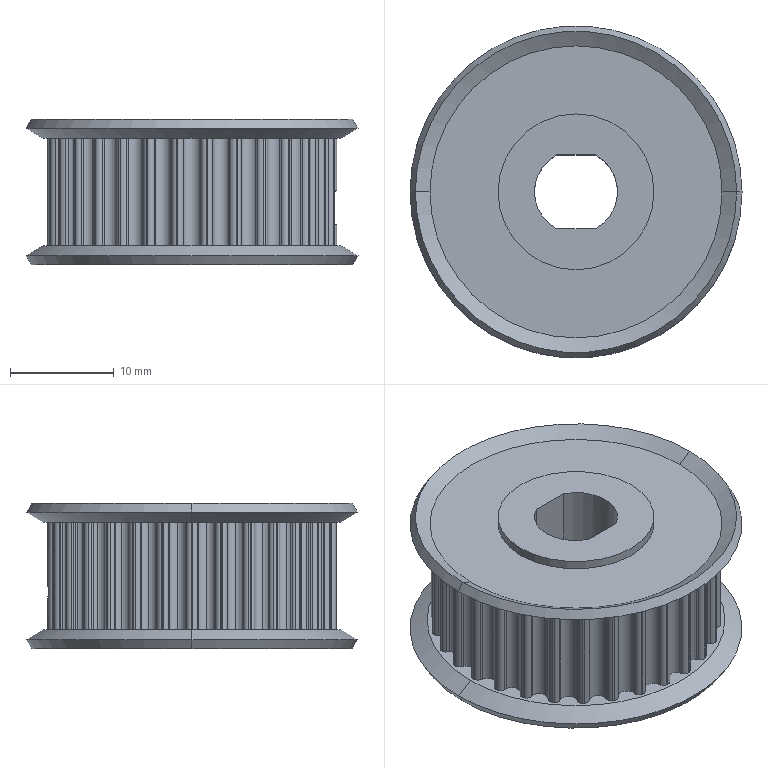Part | NX | features BREP 1 | 1 solid | 248 faces | box 31.944 x 31.944 x 14 mm | volume 6821 mm3 | cylinder 228 | cone 12 | plane 8 | commonest cylinder face diameters 1.02 x76 3.04 x66 1.7 x41 27.89 x34 3.3 x4 15 x4